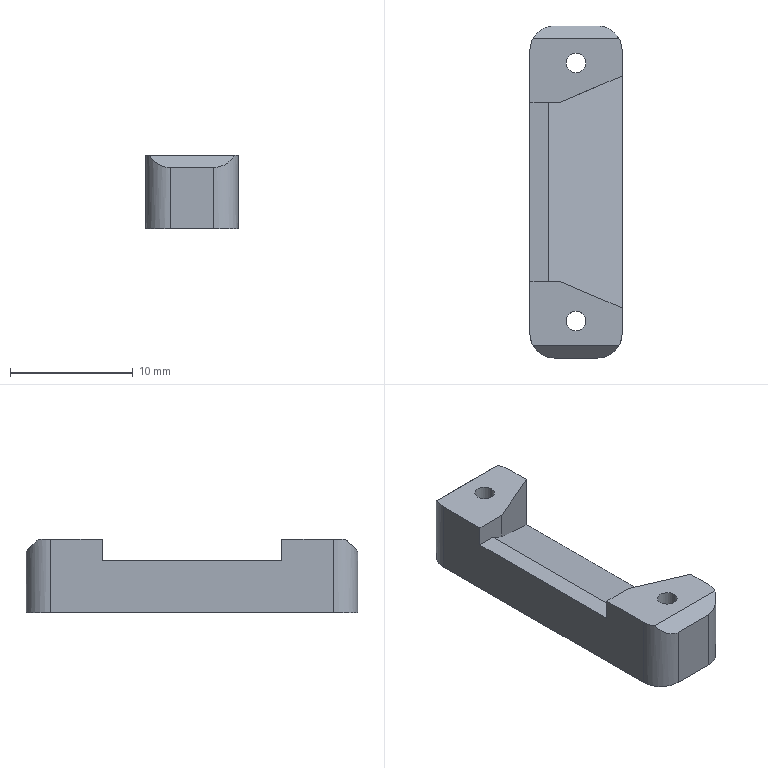Part | NX | 1 solid | 23 faces | box 7.5 x 27 x 6 mm | volume 816.193 mm3 | plane 15 | cylinder 8 | commonest cylinder face diameters 1.6 x4 4 x4
STEP:
#1=CARTESIAN_POINT('',(0.,23.,-6.5));
#2=VERTEX_POINT('',#1);
#3=CARTESIAN_POINT('',(2.,25.,-6.5));
#4=VERTEX_POINT('',#3);
#5=CARTESIAN_POINT('',(2.,23.,-6.5));
#6=DIRECTION('',(0.,0.,-1.));
#7=DIRECTION('',(1.,0.,0.));
#8=AXIS2_PLACEMENT_3D('',#5,#6,#7);
#9=CIRCLE('',#8,2.);
#10=EDGE_CURVE('',#2,#4,#9,.T.);
#11=ORIENTED_EDGE('',*,*,#10,.F.);
#12=CARTESIAN_POINT('',(0.,23.,-0.5));
#13=VERTEX_POINT('',#12);
#14=CARTESIAN_POINT('',(0.,23.,-6.5));
#15=DIRECTION('',(0.,0.,-1.));
#16=VECTOR('',#15,1000.);
#17=LINE('',#14,#16);
#18=EDGE_CURVE('',#13,#2,#17,.T.);
#19=ORIENTED_EDGE('',*,*,#18,.F.);
#20=CARTESIAN_POINT('',(0.2679,24.,-0.5));
#21=VERTEX_POINT('',#20);
#22=CARTESIAN_POINT('',(2.,23.,-0.5));
#23=DIRECTION('',(0.,0.,1.));
#24=DIRECTION('',(1.,0.,0.));
#25=AXIS2_PLACEMENT_3D('',#22,#23,#24);
#26=CIRCLE('',#25,2.);
#27=EDGE_CURVE('',#21,#13,#26,.T.);
#28=ORIENTED_EDGE('',*,*,#27,.F.);
#29=CARTESIAN_POINT('',(2.,25.,-1.5));
#30=VERTEX_POINT('',#29);
#31=CARTESIAN_POINT('',(2.,25.,-1.5));
#32=CARTESIAN_POINT('',(1.268,25.,-1.5));
#33=CARTESIAN_POINT('',(0.634,24.634,-1.134));
#34=CARTESIAN_POINT('',(0.2679,24.,-0.5));
#35=(BOUNDED_CURVE()B_SPLINE_CURVE(3,(#31,#32,#33,#34),.UNSPECIFIED.,.F.,.F.)B_SPLINE_CURVE_WITH_KNOTS((4,4),(3.142,4.189),.UNSPECIFIED.)CURVE()GEOMETRIC_REPRESENTATION_ITEM()RATIONAL_B_SPLINE_CURVE((1.,0.9107,0.9107,1.))REPRESENTATION_ITEM(''));
#36=EDGE_CURVE('',#30,#21,#35,.T.);
#37=ORIENTED_EDGE('',*,*,#36,.F.);
#38=CARTESIAN_POINT('',(2.,25.,-14.262));
#39=DIRECTION('',(0.,0.,1.));
#40=VECTOR('',#39,1000.);
#41=LINE('',#38,#40);
#42=EDGE_CURVE('',#4,#30,#41,.T.);
#43=ORIENTED_EDGE('',*,*,#42,.F.);
#44=EDGE_LOOP('',(#11,#19,#28,#37,#43));
#45=FACE_BOUND('',#44,.T.);
#46=CARTESIAN_POINT('',(2.,23.,-14.262));
#47=DIRECTION('',(0.,0.,1.));
#48=DIRECTION('',(1.,0.,0.));
#49=AXIS2_PLACEMENT_3D('',#46,#47,#48);
#50=CYLINDRICAL_SURFACE('',#49,2.);
#51=ADVANCED_FACE('',(#45),#50,.T.);
#52=CARTESIAN_POINT('',(2.,-2.,-6.5));
#53=VERTEX_POINT('',#52);
#54=CARTESIAN_POINT('',(0.,0.,-6.5));
#55=VERTEX_POINT('',#54);
#56=CARTESIAN_POINT('',(2.,0.,-6.5));
#57=DIRECTION('',(0.,0.,-1.));
#58=DIRECTION('',(1.,0.,0.));
#59=AXIS2_PLACEMENT_3D('',#56,#57,#58);
#60=CIRCLE('',#59,2.);
#61=EDGE_CURVE('',#53,#55,#60,.T.);
#62=ORIENTED_EDGE('',*,*,#61,.F.);
#63=CARTESIAN_POINT('',(2.,-2.,-1.5));
#64=VERTEX_POINT('',#63);
#65=CARTESIAN_POINT('',(2.,-2.,-14.262));
#66=DIRECTION('',(0.,0.,-1.));
#67=VECTOR('',#66,1000.);
#68=LINE('',#65,#67);
#69=EDGE_CURVE('',#64,#53,#68,.T.);
#70=ORIENTED_EDGE('',*,*,#69,.F.);
#71=CARTESIAN_POINT('',(0.2679,-1.,-0.5));
#72=VERTEX_POINT('',#71);
#73=CARTESIAN_POINT('',(0.2679,-1.,-0.5));
#74=CARTESIAN_POINT('',(0.634,-1.634,-1.134));
#75=CARTESIAN_POINT('',(1.268,-2.,-1.5));
#76=CARTESIAN_POINT('',(2.,-2.,-1.5));
#77=(BOUNDED_CURVE()B_SPLINE_CURVE(3,(#73,#74,#75,#76),.UNSPECIFIED.,.F.,.F.)B_SPLINE_CURVE_WITH_KNOTS((4,4),(2.094,3.142),.UNSPECIFIED.)CURVE()GEOMETRIC_REPRESENTATION_ITEM()RATIONAL_B_SPLINE_CURVE((1.,0.9107,0.9107,1.))REPRESENTATION_ITEM(''));
#78=EDGE_CURVE('',#72,#64,#77,.T.);
#79=ORIENTED_EDGE('',*,*,#78,.F.);
#80=CARTESIAN_POINT('',(0.,0.,-0.5));
#81=VERTEX_POINT('',#80);
#82=CARTESIAN_POINT('',(2.,0.,-0.5));
#83=DIRECTION('',(0.,0.,1.));
#84=DIRECTION('',(1.,0.,0.));
#85=AXIS2_PLACEMENT_3D('',#82,#83,#84);
#86=CIRCLE('',#85,2.);
#87=EDGE_CURVE('',#81,#72,#86,.T.);
#88=ORIENTED_EDGE('',*,*,#87,.F.);
#89=CARTESIAN_POINT('',(0.,0.,-6.5));
#90=DIRECTION('',(0.,0.,1.));
#91=VECTOR('',#90,1000.);
#92=LINE('',#89,#91);
#93=EDGE_CURVE('',#55,#81,#92,.T.);
#94=ORIENTED_EDGE('',*,*,#93,.F.);
#95=EDGE_LOOP('',(#62,#70,#79,#88,#94));
#96=FACE_BOUND('',#95,.T.);
#97=CARTESIAN_POINT('',(2.,0.,-6.5));
#98=DIRECTION('',(0.,0.,1.));
#99=DIRECTION('',(1.,0.,0.));
#100=AXIS2_PLACEMENT_3D('',#97,#98,#99);
#101=CYLINDRICAL_SURFACE('',#100,2.);
#102=ADVANCED_FACE('',(#96),#101,.T.);
#103=CARTESIAN_POINT('',(7.5,0.,-6.5));
#104=VERTEX_POINT('',#103);
#105=CARTESIAN_POINT('',(5.5,-2.,-6.5));
#106=VERTEX_POINT('',#105);
#107=CARTESIAN_POINT('',(5.5,0.,-6.5));
#108=DIRECTION('',(0.,0.,-1.));
#109=DIRECTION('',(1.,0.,0.));
#110=AXIS2_PLACEMENT_3D('',#107,#108,#109);
#111=CIRCLE('',#110,2.);
#112=EDGE_CURVE('',#104,#106,#111,.T.);
#113=ORIENTED_EDGE('',*,*,#112,.F.);
#114=CARTESIAN_POINT('',(7.5,0.,-0.5));
#115=VERTEX_POINT('',#114);
#116=CARTESIAN_POINT('',(7.5,0.,-6.5));
#117=DIRECTION('',(0.,0.,-1.));
#118=VECTOR('',#117,1000.);
#119=LINE('',#116,#118);
#120=EDGE_CURVE('',#115,#104,#119,.T.);
#121=ORIENTED_EDGE('',*,*,#120,.F.);
#122=CARTESIAN_POINT('',(7.232,-1.,-0.5));
#123=VERTEX_POINT('',#122);
#124=CARTESIAN_POINT('',(5.5,0.,-0.5));
#125=DIRECTION('',(0.,0.,1.));
#126=DIRECTION('',(1.,0.,0.));
#127=AXIS2_PLACEMENT_3D('',#124,#125,#126);
#128=CIRCLE('',#127,2.);
#129=EDGE_CURVE('',#123,#115,#128,.T.);
#130=ORIENTED_EDGE('',*,*,#129,.F.);
#131=CARTESIAN_POINT('',(5.5,-2.,-1.5));
#132=VERTEX_POINT('',#131);
#133=CARTESIAN_POINT('',(5.5,-2.,-1.5));
#134=CARTESIAN_POINT('',(6.232,-2.,-1.5));
#135=CARTESIAN_POINT('',(6.866,-1.634,-1.134));
#136=CARTESIAN_POINT('',(7.232,-1.,-0.5));
#137=(BOUNDED_CURVE()B_SPLINE_CURVE(3,(#133,#134,#135,#136),.UNSPECIFIED.,.F.,.F.)B_SPLINE_CURVE_WITH_KNOTS((4,4),(3.142,4.189),.UNSPECIFIED.)CURVE()GEOMETRIC_REPRESENTATION_ITEM()RATIONAL_B_SPLINE_CURVE((1.,0.9107,0.9107,1.))REPRESENTATION_ITEM(''));
#138=EDGE_CURVE('',#132,#123,#137,.T.);
#139=ORIENTED_EDGE('',*,*,#138,.F.);
#140=CARTESIAN_POINT('',(5.5,-2.,-14.262));
#141=DIRECTION('',(0.,0.,1.));
#142=VECTOR('',#141,1000.);
#143=LINE('',#140,#142);
#144=EDGE_CURVE('',#106,#132,#143,.T.);
#145=ORIENTED_EDGE('',*,*,#144,.F.);
#146=EDGE_LOOP('',(#113,#121,#130,#139,#145));
#147=FACE_BOUND('',#146,.T.);
#148=CARTESIAN_POINT('',(5.5,0.,-14.262));
#149=DIRECTION('',(0.,0.,1.));
#150=DIRECTION('',(1.,0.,0.));
#151=AXIS2_PLACEMENT_3D('',#148,#149,#150);
#152=CYLINDRICAL_SURFACE('',#151,2.);
#153=ADVANCED_FACE('',(#147),#152,.T.);
#154=CARTESIAN_POINT('',(5.5,25.,-6.5));
#155=VERTEX_POINT('',#154);
#156=CARTESIAN_POINT('',(7.5,23.,-6.5));
#157=VERTEX_POINT('',#156);
#158=CARTESIAN_POINT('',(5.5,23.,-6.5));
#159=DIRECTION('',(0.,0.,-1.));
#160=DIRECTION('',(1.,0.,0.));
#161=AXIS2_PLACEMENT_3D('',#158,#159,#160);
#162=CIRCLE('',#161,2.);
#163=EDGE_CURVE('',#155,#157,#162,.T.);
#164=ORIENTED_EDGE('',*,*,#163,.F.);
#165=CARTESIAN_POINT('',(5.5,25.,-1.5));
#166=VERTEX_POINT('',#165);
#167=CARTESIAN_POINT('',(5.5,25.,-14.262));
#168=DIRECTION('',(0.,0.,-1.));
#169=VECTOR('',#168,1000.);
#170=LINE('',#167,#169);
#171=EDGE_CURVE('',#166,#155,#170,.T.);
#172=ORIENTED_EDGE('',*,*,#171,.F.);
#173=CARTESIAN_POINT('',(7.232,24.,-0.5));
#174=VERTEX_POINT('',#173);
#175=CARTESIAN_POINT('',(7.232,24.,-0.5));
#176=CARTESIAN_POINT('',(6.866,24.634,-1.134));
#177=CARTESIAN_POINT('',(6.232,25.,-1.5));
#178=CARTESIAN_POINT('',(5.5,25.,-1.5));
#179=(BOUNDED_CURVE()B_SPLINE_CURVE(3,(#175,#176,#177,#178),.UNSPECIFIED.,.F.,.F.)B_SPLINE_CURVE_WITH_KNOTS((4,4),(2.094,3.142),.UNSPECIFIED.)CURVE()GEOMETRIC_REPRESENTATION_ITEM()RATIONAL_B_SPLINE_CURVE((1.,0.9107,0.9107,1.))REPRESENTATION_ITEM(''));
#180=EDGE_CURVE('',#174,#166,#179,.T.);
#181=ORIENTED_EDGE('',*,*,#180,.F.);
#182=CARTESIAN_POINT('',(7.5,23.,-0.5));
#183=VERTEX_POINT('',#182);
#184=CARTESIAN_POINT('',(5.5,23.,-0.5));
#185=DIRECTION('',(0.,0.,1.));
#186=DIRECTION('',(1.,0.,0.));
#187=AXIS2_PLACEMENT_3D('',#184,#185,#186);
#188=CIRCLE('',#187,2.);
#189=EDGE_CURVE('',#183,#174,#188,.T.);
#190=ORIENTED_EDGE('',*,*,#189,.F.);
#191=CARTESIAN_POINT('',(7.5,23.,-6.5));
#192=DIRECTION('',(0.,0.,1.));
#193=VECTOR('',#192,1000.);
#194=LINE('',#191,#193);
#195=EDGE_CURVE('',#157,#183,#194,.T.);
#196=ORIENTED_EDGE('',*,*,#195,.F.);
#197=EDGE_LOOP('',(#164,#172,#181,#190,#196));
#198=FACE_BOUND('',#197,.T.);
#199=CARTESIAN_POINT('',(5.5,23.,-6.5));
#200=DIRECTION('',(0.,0.,1.));
#201=DIRECTION('',(1.,0.,0.));
#202=AXIS2_PLACEMENT_3D('',#199,#200,#201);
#203=CYLINDRICAL_SURFACE('',#202,2.);
#204=ADVANCED_FACE('',(#198),#203,.T.);
#205=CARTESIAN_POINT('',(4.55,22.,-0.5));
#206=VERTEX_POINT('',#205);
#207=CARTESIAN_POINT('',(4.55,22.,-6.5));
#208=VERTEX_POINT('',#207);
#209=CARTESIAN_POINT('',(4.55,22.,-6.5));
#210=DIRECTION('',(0.,0.,-1.));
#211=VECTOR('',#210,1000.);
#212=LINE('',#209,#211);
#213=EDGE_CURVE('',#206,#208,#212,.T.);
#214=ORIENTED_EDGE('',*,*,#213,.F.);
#215=CARTESIAN_POINT('',(2.95,22.,-0.5));
#216=VERTEX_POINT('',#215);
#217=CARTESIAN_POINT('',(3.75,22.,-0.5));
#218=DIRECTION('',(0.,0.,1.));
#219=DIRECTION('',(1.,0.,0.));
#220=AXIS2_PLACEMENT_3D('',#217,#218,#219);
#221=CIRCLE('',#220,0.8);
#222=EDGE_CURVE('',#206,#216,#221,.T.);
#223=ORIENTED_EDGE('',*,*,#222,.T.);
#224=CARTESIAN_POINT('',(2.95,22.,-6.5));
#225=VERTEX_POINT('',#224);
#226=CARTESIAN_POINT('',(2.95,22.,-6.5));
#227=DIRECTION('',(0.,0.,-1.));
#228=VECTOR('',#227,1000.);
#229=LINE('',#226,#228);
#230=EDGE_CURVE('',#216,#225,#229,.T.);
#231=ORIENTED_EDGE('',*,*,#230,.T.);
#232=CARTESIAN_POINT('',(3.75,22.,-6.5));
#233=DIRECTION('',(0.,0.,-1.));
#234=DIRECTION('',(-1.,0.,0.));
#235=AXIS2_PLACEMENT_3D('',#232,#233,#234);
#236=CIRCLE('',#235,0.8);
#237=EDGE_CURVE('',#225,#208,#236,.T.);
#238=ORIENTED_EDGE('',*,*,#237,.T.);
#239=EDGE_LOOP('',(#214,#223,#231,#238));
#240=FACE_BOUND('',#239,.T.);
#241=CARTESIAN_POINT('',(3.75,22.,-6.5));
#242=DIRECTION('',(0.,0.,-1.));
#243=DIRECTION('',(-1.,0.,0.));
#244=AXIS2_PLACEMENT_3D('',#241,#242,#243);
#245=CYLINDRICAL_SURFACE('',#244,0.8);
#246=ADVANCED_FACE('',(#240),#245,.F.);
#247=CARTESIAN_POINT('',(4.55,1.,-0.5));
#248=VERTEX_POINT('',#247);
#249=CARTESIAN_POINT('',(4.55,1.,-6.5));
#250=VERTEX_POINT('',#249);
#251=CARTESIAN_POINT('',(4.55,1.,-6.5));
#252=DIRECTION('',(0.,0.,-1.));
#253=VECTOR('',#252,1000.);
#254=LINE('',#251,#253);
#255=EDGE_CURVE('',#248,#250,#254,.T.);
#256=ORIENTED_EDGE('',*,*,#255,.F.);
#257=CARTESIAN_POINT('',(2.95,1.,-0.5));
#258=VERTEX_POINT('',#257);
#259=CARTESIAN_POINT('',(3.75,1.,-0.5));
#260=DIRECTION('',(0.,0.,1.));
#261=DIRECTION('',(1.,0.,0.));
#262=AXIS2_PLACEMENT_3D('',#259,#260,#261);
#263=CIRCLE('',#262,0.8);
#264=EDGE_CURVE('',#248,#258,#263,.T.);
#265=ORIENTED_EDGE('',*,*,#264,.T.);
#266=CARTESIAN_POINT('',(2.95,1.,-6.5));
#267=VERTEX_POINT('',#266);
#268=CARTESIAN_POINT('',(2.95,1.,-6.5));
#269=DIRECTION('',(0.,0.,-1.));
#270=VECTOR('',#269,1000.);
#271=LINE('',#268,#270);
#272=EDGE_CURVE('',#258,#267,#271,.T.);
#273=ORIENTED_EDGE('',*,*,#272,.T.);
#274=CARTESIAN_POINT('',(3.75,1.,-6.5));
#275=DIRECTION('',(0.,0.,-1.));
#276=DIRECTION('',(-1.,0.,0.));
#277=AXIS2_PLACEMENT_3D('',#274,#275,#276);
#278=CIRCLE('',#277,0.8);
#279=EDGE_CURVE('',#267,#250,#278,.T.);
#280=ORIENTED_EDGE('',*,*,#279,.T.);
#281=EDGE_LOOP('',(#256,#265,#273,#280));
#282=FACE_BOUND('',#281,.T.);
#283=CARTESIAN_POINT('',(3.75,1.,-6.5));
#284=DIRECTION('',(0.,0.,-1.));
#285=DIRECTION('',(-1.,0.,0.));
#286=AXIS2_PLACEMENT_3D('',#283,#284,#285);
#287=CYLINDRICAL_SURFACE('',#286,0.8);
#288=ADVANCED_FACE('',(#282),#287,.F.);
#289=CARTESIAN_POINT('',(7.5,2.057,-4.998));
#290=VERTEX_POINT('',#289);
#291=CARTESIAN_POINT('',(2.5,4.2,-2.666));
#292=VERTEX_POINT('',#291);
#293=CARTESIAN_POINT('',(6.569,2.456,-4.564));
#294=DIRECTION('',(-0.8448,0.3621,0.3939));
#295=VECTOR('',#294,1000.);
#296=LINE('',#293,#295);
#297=EDGE_CURVE('',#290,#292,#296,.T.);
#298=ORIENTED_EDGE('',*,*,#297,.F.);
#299=CARTESIAN_POINT('',(7.5,20.943,-4.998));
#300=VERTEX_POINT('',#299);
#301=CARTESIAN_POINT('',(7.5,2.057,-4.998));
#302=DIRECTION('',(0.,-1.,0.));
#303=VECTOR('',#302,1000.);
#304=LINE('',#301,#303);
#305=EDGE_CURVE('',#300,#290,#304,.T.);
#306=ORIENTED_EDGE('',*,*,#305,.F.);
#307=CARTESIAN_POINT('',(2.5,18.8,-2.666));
#308=VERTEX_POINT('',#307);
#309=CARTESIAN_POINT('',(2.345,18.733,-2.594));
#310=DIRECTION('',(0.8448,0.3621,-0.3939));
#311=VECTOR('',#310,1000.);
#312=LINE('',#309,#311);
#313=EDGE_CURVE('',#308,#300,#312,.T.);
#314=ORIENTED_EDGE('',*,*,#313,.F.);
#315=CARTESIAN_POINT('',(1.5,18.8,-2.2));
#316=VERTEX_POINT('',#315);
#317=CARTESIAN_POINT('',(0.2679,18.8,-1.625));
#318=DIRECTION('',(0.9063,0.,-0.4226));
#319=VECTOR('',#318,1000.);
#320=LINE('',#317,#319);
#321=EDGE_CURVE('',#316,#308,#320,.T.);
#322=ORIENTED_EDGE('',*,*,#321,.F.);
#323=CARTESIAN_POINT('',(1.5,4.2,-2.2));
#324=VERTEX_POINT('',#323);
#325=CARTESIAN_POINT('',(1.5,20.943,-2.2));
#326=DIRECTION('',(0.,1.,0.));
#327=VECTOR('',#326,1000.);
#328=LINE('',#325,#327);
#329=EDGE_CURVE('',#324,#316,#328,.T.);
#330=ORIENTED_EDGE('',*,*,#329,.F.);
#331=CARTESIAN_POINT('',(2.321,4.2,-2.583));
#332=DIRECTION('',(-0.9063,0.,0.4226));
#333=VECTOR('',#332,1000.);
#334=LINE('',#331,#333);
#335=EDGE_CURVE('',#292,#324,#334,.T.);
#336=ORIENTED_EDGE('',*,*,#335,.F.);
#337=EDGE_LOOP('',(#298,#306,#314,#322,#330,#336));
#338=FACE_BOUND('',#337,.T.);
#339=CARTESIAN_POINT('',(1.5,0.,-2.2));
#340=DIRECTION('',(0.4226,0.,0.9063));
#341=DIRECTION('',(0.,-1.,0.));
#342=AXIS2_PLACEMENT_3D('',#339,#340,#341);
#343=PLANE('',#342);
#344=ADVANCED_FACE('',(#338),#343,.T.);
#345=CARTESIAN_POINT('',(0.,-2.,-1.5));
#346=DIRECTION('',(-1.,0.,0.));
#347=VECTOR('',#346,1000.);
#348=LINE('',#345,#347);
#349=EDGE_CURVE('',#132,#64,#348,.T.);
#350=ORIENTED_EDGE('',*,*,#349,.F.);
#351=ORIENTED_EDGE('',*,*,#138,.T.);
#352=CARTESIAN_POINT('',(0.,-1.,-0.5));
#353=DIRECTION('',(1.,0.,0.));
#354=VECTOR('',#353,1000.);
#355=LINE('',#352,#354);
#356=EDGE_CURVE('',#72,#123,#355,.T.);
#357=ORIENTED_EDGE('',*,*,#356,.F.);
#358=ORIENTED_EDGE('',*,*,#78,.T.);
#359=EDGE_LOOP('',(#350,#351,#357,#358));
#360=FACE_BOUND('',#359,.T.);
#361=CARTESIAN_POINT('',(0.,-1.,-0.5));
#362=DIRECTION('',(0.,0.7071,-0.7071));
#363=DIRECTION('',(1.,0.,0.));
#364=AXIS2_PLACEMENT_3D('',#361,#362,#363);
#365=PLANE('',#364);
#366=ADVANCED_FACE('',(#360),#365,.F.);
#367=CARTESIAN_POINT('',(0.,24.,-0.5));
#368=DIRECTION('',(-1.,0.,0.));
#369=VECTOR('',#368,1000.);
#370=LINE('',#367,#369);
#371=EDGE_CURVE('',#174,#21,#370,.T.);
#372=ORIENTED_EDGE('',*,*,#371,.F.);
#373=ORIENTED_EDGE('',*,*,#180,.T.);
#374=CARTESIAN_POINT('',(7.5,25.,-1.5));
#375=DIRECTION('',(1.,0.,0.));
#376=VECTOR('',#375,1000.);
#377=LINE('',#374,#376);
#378=EDGE_CURVE('',#30,#166,#377,.T.);
#379=ORIENTED_EDGE('',*,*,#378,.F.);
#380=ORIENTED_EDGE('',*,*,#36,.T.);
#381=EDGE_LOOP('',(#372,#373,#379,#380));
#382=FACE_BOUND('',#381,.T.);
#383=CARTESIAN_POINT('',(0.,24.,-0.5));
#384=DIRECTION('',(0.,-0.7071,-0.7071));
#385=DIRECTION('',(-1.,0.,0.));
#386=AXIS2_PLACEMENT_3D('',#383,#384,#385);
#387=PLANE('',#386);
#388=ADVANCED_FACE('',(#382),#387,.F.);
#389=CARTESIAN_POINT('',(0.,4.2,-2.2));
#390=VERTEX_POINT('',#389);
#391=CARTESIAN_POINT('',(2.5,4.2,-2.2));
#392=DIRECTION('',(1.,0.,0.));
#393=VECTOR('',#392,1000.);
#394=LINE('',#391,#393);
#395=EDGE_CURVE('',#390,#324,#394,.T.);
#396=ORIENTED_EDGE('',*,*,#395,.T.);
#397=ORIENTED_EDGE('',*,*,#329,.T.);
#398=CARTESIAN_POINT('',(0.,18.8,-2.2));
#399=VERTEX_POINT('',#398);
#400=CARTESIAN_POINT('',(0.,18.8,-2.2));
#401=DIRECTION('',(-1.,0.,0.));
#402=VECTOR('',#401,1000.);
#403=LINE('',#400,#402);
#404=EDGE_CURVE('',#316,#399,#403,.T.);
#405=ORIENTED_EDGE('',*,*,#404,.T.);
#406=CARTESIAN_POINT('',(0.,4.2,-2.2));
#407=DIRECTION('',(0.,-1.,0.));
#408=VECTOR('',#407,1000.);
#409=LINE('',#406,#408);
#410=EDGE_CURVE('',#399,#390,#409,.T.);
#411=ORIENTED_EDGE('',*,*,#410,.T.);
#412=EDGE_LOOP('',(#396,#397,#405,#411));
#413=FACE_BOUND('',#412,.T.);
#414=CARTESIAN_POINT('',(0.,0.,-2.2));
#415=DIRECTION('',(0.,0.,-1.));
#416=DIRECTION('',(-1.,0.,0.));
#417=AXIS2_PLACEMENT_3D('',#414,#415,#416);
#418=PLANE('',#417);
#419=ADVANCED_FACE('',(#413),#418,.F.);
#420=CARTESIAN_POINT('',(7.5,20.943,-0.5));
#421=VERTEX_POINT('',#420);
#422=CARTESIAN_POINT('',(2.5,18.8,-0.5));
#423=VERTEX_POINT('',#422);
#424=CARTESIAN_POINT('',(2.5,18.8,-0.5));
#425=DIRECTION('',(-0.9191,-0.3939,0.));
#426=VECTOR('',#425,1000.);
#427=LINE('',#424,#426);
#428=EDGE_CURVE('',#421,#423,#427,.T.);
#429=ORIENTED_EDGE('',*,*,#428,.T.);
#430=CARTESIAN_POINT('',(2.5,18.8,-2.2));
#431=DIRECTION('',(0.,0.,1.));
#432=VECTOR('',#431,1000.);
#433=LINE('',#430,#432);
#434=EDGE_CURVE('',#308,#423,#433,.T.);
#435=ORIENTED_EDGE('',*,*,#434,.F.);
#436=ORIENTED_EDGE('',*,*,#313,.T.);
#437=CARTESIAN_POINT('',(7.5,20.943,-2.2));
#438=DIRECTION('',(0.,0.,1.));
#439=VECTOR('',#438,1000.);
#440=LINE('',#437,#439);
#441=EDGE_CURVE('',#300,#421,#440,.T.);
#442=ORIENTED_EDGE('',*,*,#441,.T.);
#443=EDGE_LOOP('',(#429,#435,#436,#442));
#444=FACE_BOUND('',#443,.T.);
#445=CARTESIAN_POINT('',(2.5,18.8,-2.2));
#446=DIRECTION('',(-0.3939,0.9191,0.));
#447=DIRECTION('',(-0.9191,-0.3939,0.));
#448=AXIS2_PLACEMENT_3D('',#445,#446,#447);
#449=PLANE('',#448);
#450=ADVANCED_FACE('',(#444),#449,.F.);
#451=CARTESIAN_POINT('',(0.,18.8,-0.5));
#452=VERTEX_POINT('',#451);
#453=CARTESIAN_POINT('',(0.,18.8,-0.5));
#454=DIRECTION('',(-1.,0.,0.));
#455=VECTOR('',#454,1000.);
#456=LINE('',#453,#455);
#457=EDGE_CURVE('',#423,#452,#456,.T.);
#458=ORIENTED_EDGE('',*,*,#457,.T.);
#459=CARTESIAN_POINT('',(0.,18.8,-2.2));
#460=DIRECTION('',(0.,0.,1.));
#461=VECTOR('',#460,1000.);
#462=LINE('',#459,#461);
#463=EDGE_CURVE('',#399,#452,#462,.T.);
#464=ORIENTED_EDGE('',*,*,#463,.F.);
#465=ORIENTED_EDGE('',*,*,#404,.F.);
#466=ORIENTED_EDGE('',*,*,#321,.T.);
#467=ORIENTED_EDGE('',*,*,#434,.T.);
#468=EDGE_LOOP('',(#458,#464,#465,#466,#467));
#469=FACE_BOUND('',#468,.T.);
#470=CARTESIAN_POINT('',(0.,18.8,-2.2));
#471=DIRECTION('',(0.,1.,0.));
#472=DIRECTION('',(0.,0.,1.));
#473=AXIS2_PLACEMENT_3D('',#470,#471,#472);
#474=PLANE('',#473);
#475=ADVANCED_FACE('',(#469),#474,.F.);
#476=CARTESIAN_POINT('',(0.,4.2,-0.5));
#477=VERTEX_POINT('',#476);
#478=CARTESIAN_POINT('',(2.5,4.2,-0.5));
#479=VERTEX_POINT('',#478);
#480=CARTESIAN_POINT('',(2.5,4.2,-0.5));
#481=DIRECTION('',(1.,0.,0.));
#482=VECTOR('',#481,1000.);
#483=LINE('',#480,#482);
#484=EDGE_CURVE('',#477,#479,#483,.T.);
#485=ORIENTED_EDGE('',*,*,#484,.T.);
#486=CARTESIAN_POINT('',(2.5,4.2,-2.2));
#487=DIRECTION('',(0.,0.,1.));
#488=VECTOR('',#487,1000.);
#489=LINE('',#486,#488);
#490=EDGE_CURVE('',#292,#479,#489,.T.);
#491=ORIENTED_EDGE('',*,*,#490,.F.);
#492=ORIENTED_EDGE('',*,*,#335,.T.);
#493=ORIENTED_EDGE('',*,*,#395,.F.);
#494=CARTESIAN_POINT('',(0.,4.2,-2.2));
#495=DIRECTION('',(0.,0.,1.));
#496=VECTOR('',#495,1000.);
#497=LINE('',#494,#496);
#498=EDGE_CURVE('',#390,#477,#497,.T.);
#499=ORIENTED_EDGE('',*,*,#498,.T.);
#500=EDGE_LOOP('',(#485,#491,#492,#493,#499));
#501=FACE_BOUND('',#500,.T.);
#502=CARTESIAN_POINT('',(2.5,4.2,-2.2));
#503=DIRECTION('',(0.,-1.,0.));
#504=DIRECTION('',(0.,0.,-1.));
#505=AXIS2_PLACEMENT_3D('',#502,#503,#504);
#506=PLANE('',#505);
#507=ADVANCED_FACE('',(#501),#506,.F.);
#508=CARTESIAN_POINT('',(7.5,2.057,-0.5));
#509=VERTEX_POINT('',#508);
#510=CARTESIAN_POINT('',(7.5,2.057,-0.5));
#511=DIRECTION('',(0.9191,-0.3939,0.));
#512=VECTOR('',#511,1000.);
#513=LINE('',#510,#512);
#514=EDGE_CURVE('',#479,#509,#513,.T.);
#515=ORIENTED_EDGE('',*,*,#514,.T.);
#516=CARTESIAN_POINT('',(7.5,2.057,-2.2));
#517=DIRECTION('',(0.,0.,1.));
#518=VECTOR('',#517,1000.);
#519=LINE('',#516,#518);
#520=EDGE_CURVE('',#290,#509,#519,.T.);
#521=ORIENTED_EDGE('',*,*,#520,.F.);
#522=ORIENTED_EDGE('',*,*,#297,.T.);
#523=ORIENTED_EDGE('',*,*,#490,.T.);
#524=EDGE_LOOP('',(#515,#521,#522,#523));
#525=FACE_BOUND('',#524,.T.);
#526=CARTESIAN_POINT('',(7.5,2.057,-2.2));
#527=DIRECTION('',(-0.3939,-0.9191,0.));
#528=DIRECTION('',(0.9191,-0.3939,0.));
#529=AXIS2_PLACEMENT_3D('',#526,#527,#528);
#530=PLANE('',#529);
#531=ADVANCED_FACE('',(#525),#530,.F.);
#532=CARTESIAN_POINT('',(0.,-2.,-6.5));
#533=DIRECTION('',(-1.,0.,0.));
#534=VECTOR('',#533,1000.);
#535=LINE('',#532,#534);
#536=EDGE_CURVE('',#106,#53,#535,.T.);
#537=ORIENTED_EDGE('',*,*,#536,.F.);
#538=ORIENTED_EDGE('',*,*,#144,.T.);
#539=ORIENTED_EDGE('',*,*,#349,.T.);
#540=ORIENTED_EDGE('',*,*,#69,.T.);
#541=EDGE_LOOP('',(#537,#538,#539,#540));
#542=FACE_BOUND('',#541,.T.);
#543=CARTESIAN_POINT('',(0.,-2.,-14.262));
#544=DIRECTION('',(0.,-1.,0.));
#545=DIRECTION('',(0.,0.,-1.));
#546=AXIS2_PLACEMENT_3D('',#543,#544,#545);
#547=PLANE('',#546);
#548=ADVANCED_FACE('',(#542),#547,.T.);
#549=ORIENTED_EDGE('',*,*,#378,.T.);
#550=ORIENTED_EDGE('',*,*,#171,.T.);
#551=CARTESIAN_POINT('',(7.5,25.,-6.5));
#552=DIRECTION('',(1.,0.,0.));
#553=VECTOR('',#552,1000.);
#554=LINE('',#551,#553);
#555=EDGE_CURVE('',#4,#155,#554,.T.);
#556=ORIENTED_EDGE('',*,*,#555,.F.);
#557=ORIENTED_EDGE('',*,*,#42,.T.);
#558=EDGE_LOOP('',(#549,#550,#556,#557));
#559=FACE_BOUND('',#558,.T.);
#560=CARTESIAN_POINT('',(7.5,25.,-14.262));
#561=DIRECTION('',(0.,1.,0.));
#562=DIRECTION('',(0.,0.,1.));
#563=AXIS2_PLACEMENT_3D('',#560,#561,#562);
#564=PLANE('',#563);
#565=ADVANCED_FACE('',(#559),#564,.T.);
#566=CARTESIAN_POINT('',(7.5,0.,-0.5));
#567=DIRECTION('',(0.,1.,0.));
#568=VECTOR('',#567,1000.);
#569=LINE('',#566,#568);
#570=EDGE_CURVE('',#421,#183,#569,.T.);
#571=ORIENTED_EDGE('',*,*,#570,.T.);
#572=ORIENTED_EDGE('',*,*,#189,.T.);
#573=ORIENTED_EDGE('',*,*,#371,.T.);
#574=ORIENTED_EDGE('',*,*,#27,.T.);
#575=CARTESIAN_POINT('',(0.,23.,-0.5));
#576=DIRECTION('',(0.,-1.,0.));
#577=VECTOR('',#576,1000.);
#578=LINE('',#575,#577);
#579=EDGE_CURVE('',#13,#452,#578,.T.);
#580=ORIENTED_EDGE('',*,*,#579,.T.);
#581=ORIENTED_EDGE('',*,*,#457,.F.);
#582=ORIENTED_EDGE('',*,*,#428,.F.);
#583=EDGE_LOOP('',(#571,#572,#573,#574,#580,#581,#582));
#584=FACE_BOUND('',#583,.T.);
#585=CARTESIAN_POINT('',(3.75,22.,-0.5));
#586=DIRECTION('',(0.,0.,1.));
#587=DIRECTION('',(1.,0.,0.));
#588=AXIS2_PLACEMENT_3D('',#585,#586,#587);
#589=CIRCLE('',#588,0.8);
#590=EDGE_CURVE('',#216,#206,#589,.T.);
#591=ORIENTED_EDGE('',*,*,#590,.F.);
#592=ORIENTED_EDGE('',*,*,#222,.F.);
#593=EDGE_LOOP('',(#591,#592));
#594=FACE_BOUND('',#593,.T.);
#595=CARTESIAN_POINT('',(0.,0.,-0.5));
#596=DIRECTION('',(0.,0.,1.));
#597=DIRECTION('',(1.,0.,0.));
#598=AXIS2_PLACEMENT_3D('',#595,#596,#597);
#599=PLANE('',#598);
#600=ADVANCED_FACE('',(#584,#594),#599,.T.);
#601=ORIENTED_EDGE('',*,*,#555,.T.);
#602=ORIENTED_EDGE('',*,*,#163,.T.);
#603=CARTESIAN_POINT('',(7.5,0.,-6.5));
#604=DIRECTION('',(0.,1.,0.));
#605=VECTOR('',#604,1000.);
#606=LINE('',#603,#605);
#607=EDGE_CURVE('',#104,#157,#606,.T.);
#608=ORIENTED_EDGE('',*,*,#607,.F.);
#609=ORIENTED_EDGE('',*,*,#112,.T.);
#610=ORIENTED_EDGE('',*,*,#536,.T.);
#611=ORIENTED_EDGE('',*,*,#61,.T.);
#612=CARTESIAN_POINT('',(0.,23.,-6.5));
#613=DIRECTION('',(0.,-1.,0.));
#614=VECTOR('',#613,1000.);
#615=LINE('',#612,#614);
#616=EDGE_CURVE('',#2,#55,#615,.T.);
#617=ORIENTED_EDGE('',*,*,#616,.F.);
#618=ORIENTED_EDGE('',*,*,#10,.T.);
#619=EDGE_LOOP('',(#601,#602,#608,#609,#610,#611,#617,#618));
#620=FACE_BOUND('',#619,.T.);
#621=ORIENTED_EDGE('',*,*,#279,.F.);
#622=CARTESIAN_POINT('',(3.75,1.,-6.5));
#623=DIRECTION('',(0.,0.,-1.));
#624=DIRECTION('',(-1.,0.,0.));
#625=AXIS2_PLACEMENT_3D('',#622,#623,#624);
#626=CIRCLE('',#625,0.8);
#627=EDGE_CURVE('',#250,#267,#626,.T.);
#628=ORIENTED_EDGE('',*,*,#627,.F.);
#629=EDGE_LOOP('',(#621,#628));
#630=FACE_BOUND('',#629,.T.);
#631=ORIENTED_EDGE('',*,*,#237,.F.);
#632=CARTESIAN_POINT('',(3.75,22.,-6.5));
#633=DIRECTION('',(0.,0.,-1.));
#634=DIRECTION('',(-1.,0.,0.));
#635=AXIS2_PLACEMENT_3D('',#632,#633,#634);
#636=CIRCLE('',#635,0.8);
#637=EDGE_CURVE('',#208,#225,#636,.T.);
#638=ORIENTED_EDGE('',*,*,#637,.F.);
#639=EDGE_LOOP('',(#631,#638));
#640=FACE_BOUND('',#639,.T.);
#641=CARTESIAN_POINT('',(0.,0.,-6.5));
#642=DIRECTION('',(0.,0.,1.));
#643=DIRECTION('',(1.,0.,0.));
#644=AXIS2_PLACEMENT_3D('',#641,#642,#643);
#645=PLANE('',#644);
#646=ADVANCED_FACE('',(#620,#630,#640),#645,.F.);
#647=ORIENTED_EDGE('',*,*,#607,.T.);
#648=ORIENTED_EDGE('',*,*,#195,.T.);
#649=ORIENTED_EDGE('',*,*,#570,.F.);
#650=ORIENTED_EDGE('',*,*,#441,.F.);
#651=ORIENTED_EDGE('',*,*,#305,.T.);
#652=ORIENTED_EDGE('',*,*,#520,.T.);
#653=CARTESIAN_POINT('',(7.5,0.,-0.5));
#654=DIRECTION('',(0.,1.,0.));
#655=VECTOR('',#654,1000.);
#656=LINE('',#653,#655);
#657=EDGE_CURVE('',#115,#509,#656,.T.);
#658=ORIENTED_EDGE('',*,*,#657,.F.);
#659=ORIENTED_EDGE('',*,*,#120,.T.);
#660=EDGE_LOOP('',(#647,#648,#649,#650,#651,#652,#658,#659));
#661=FACE_BOUND('',#660,.T.);
#662=CARTESIAN_POINT('',(7.5,0.,-6.5));
#663=DIRECTION('',(1.,0.,0.));
#664=DIRECTION('',(0.,0.,-1.));
#665=AXIS2_PLACEMENT_3D('',#662,#663,#664);
#666=PLANE('',#665);
#667=ADVANCED_FACE('',(#661),#666,.T.);
#668=ORIENTED_EDGE('',*,*,#616,.T.);
#669=ORIENTED_EDGE('',*,*,#93,.T.);
#670=CARTESIAN_POINT('',(0.,23.,-0.5));
#671=DIRECTION('',(0.,-1.,0.));
#672=VECTOR('',#671,1000.);
#673=LINE('',#670,#672);
#674=EDGE_CURVE('',#477,#81,#673,.T.);
#675=ORIENTED_EDGE('',*,*,#674,.F.);
#676=ORIENTED_EDGE('',*,*,#498,.F.);
#677=ORIENTED_EDGE('',*,*,#410,.F.);
#678=ORIENTED_EDGE('',*,*,#463,.T.);
#679=ORIENTED_EDGE('',*,*,#579,.F.);
#680=ORIENTED_EDGE('',*,*,#18,.T.);
#681=EDGE_LOOP('',(#668,#669,#675,#676,#677,#678,#679,#680));
#682=FACE_BOUND('',#681,.T.);
#683=CARTESIAN_POINT('',(0.,23.,-6.5));
#684=DIRECTION('',(-1.,0.,0.));
#685=DIRECTION('',(0.,-1.,0.));
#686=AXIS2_PLACEMENT_3D('',#683,#684,#685);
#687=PLANE('',#686);
#688=ADVANCED_FACE('',(#682),#687,.T.);
#689=ORIENTED_EDGE('',*,*,#356,.T.);
#690=ORIENTED_EDGE('',*,*,#129,.T.);
#691=ORIENTED_EDGE('',*,*,#657,.T.);
#692=ORIENTED_EDGE('',*,*,#514,.F.);
#693=ORIENTED_EDGE('',*,*,#484,.F.);
#694=ORIENTED_EDGE('',*,*,#674,.T.);
#695=ORIENTED_EDGE('',*,*,#87,.T.);
#696=EDGE_LOOP('',(#689,#690,#691,#692,#693,#694,#695));
#697=FACE_BOUND('',#696,.T.);
#698=CARTESIAN_POINT('',(3.75,1.,-0.5));
#699=DIRECTION('',(0.,0.,1.));
#700=DIRECTION('',(1.,0.,0.));
#701=AXIS2_PLACEMENT_3D('',#698,#699,#700);
#702=CIRCLE('',#701,0.8);
#703=EDGE_CURVE('',#258,#248,#702,.T.);
#704=ORIENTED_EDGE('',*,*,#703,.F.);
#705=ORIENTED_EDGE('',*,*,#264,.F.);
#706=EDGE_LOOP('',(#704,#705));
#707=FACE_BOUND('',#706,.T.);
#708=CARTESIAN_POINT('',(0.,0.,-0.5));
#709=DIRECTION('',(0.,0.,1.));
#710=DIRECTION('',(1.,0.,0.));
#711=AXIS2_PLACEMENT_3D('',#708,#709,#710);
#712=PLANE('',#711);
#713=ADVANCED_FACE('',(#697,#707),#712,.T.);
#714=ORIENTED_EDGE('',*,*,#703,.T.);
#715=ORIENTED_EDGE('',*,*,#255,.T.);
#716=ORIENTED_EDGE('',*,*,#627,.T.);
#717=ORIENTED_EDGE('',*,*,#272,.F.);
#718=EDGE_LOOP('',(#714,#715,#716,#717));
#719=FACE_BOUND('',#718,.T.);
#720=CARTESIAN_POINT('',(3.75,1.,-6.5));
#721=DIRECTION('',(0.,0.,-1.));
#722=DIRECTION('',(-1.,0.,0.));
#723=AXIS2_PLACEMENT_3D('',#720,#721,#722);
#724=CYLINDRICAL_SURFACE('',#723,0.8);
#725=ADVANCED_FACE('',(#719),#724,.F.);
#726=ORIENTED_EDGE('',*,*,#590,.T.);
#727=ORIENTED_EDGE('',*,*,#213,.T.);
#728=ORIENTED_EDGE('',*,*,#637,.T.);
#729=ORIENTED_EDGE('',*,*,#230,.F.);
#730=EDGE_LOOP('',(#726,#727,#728,#729));
#731=FACE_BOUND('',#730,.T.);
#732=CARTESIAN_POINT('',(3.75,22.,-6.5));
#733=DIRECTION('',(0.,0.,-1.));
#734=DIRECTION('',(-1.,0.,0.));
#735=AXIS2_PLACEMENT_3D('',#732,#733,#734);
#736=CYLINDRICAL_SURFACE('',#735,0.8);
#737=ADVANCED_FACE('',(#731),#736,.F.);
#738=CLOSED_SHELL('',(#51,#102,#153,#204,#246,#288,#344,#366,#388,#419,#450,#475,#507,#531,#548,#565,#600,#646,#667,#688,#713,#725,#737));
#739=MANIFOLD_SOLID_BREP('',#738);
#740=(LENGTH_UNIT()NAMED_UNIT(*)SI_UNIT(.MILLI.,.METRE.));
#741=UNCERTAINTY_MEASURE_WITH_UNIT(LENGTH_MEASURE(0.00001),#740,'','');
#742=(NAMED_UNIT(*)PLANE_ANGLE_UNIT()SI_UNIT($,.RADIAN.));
#743=(NAMED_UNIT(*)SI_UNIT($,.STERADIAN.)SOLID_ANGLE_UNIT());
#744=(GEOMETRIC_REPRESENTATION_CONTEXT(3)GLOBAL_UNCERTAINTY_ASSIGNED_CONTEXT((#741))GLOBAL_UNIT_ASSIGNED_CONTEXT((#740,#742,#743))REPRESENTATION_CONTEXT('',''));
#745=ADVANCED_BREP_SHAPE_REPRESENTATION('',(#739),#744);